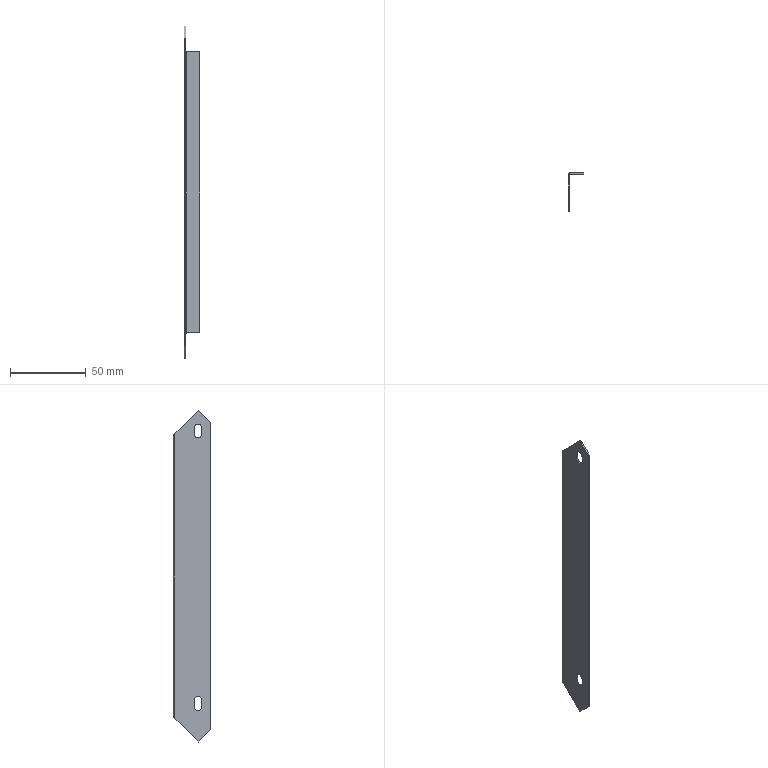Part | STEP file | RJWD-DY-0102_X2_5DE667DC95E8_26 | 1 solid | 28 faces | box 10 x 25 x 219.358 mm | volume 6666 mm3 | plane 20 | cylinder 6 | spline 2 | commonest cylinder face diameters 5 x4 0.4 x1 2.4 x1